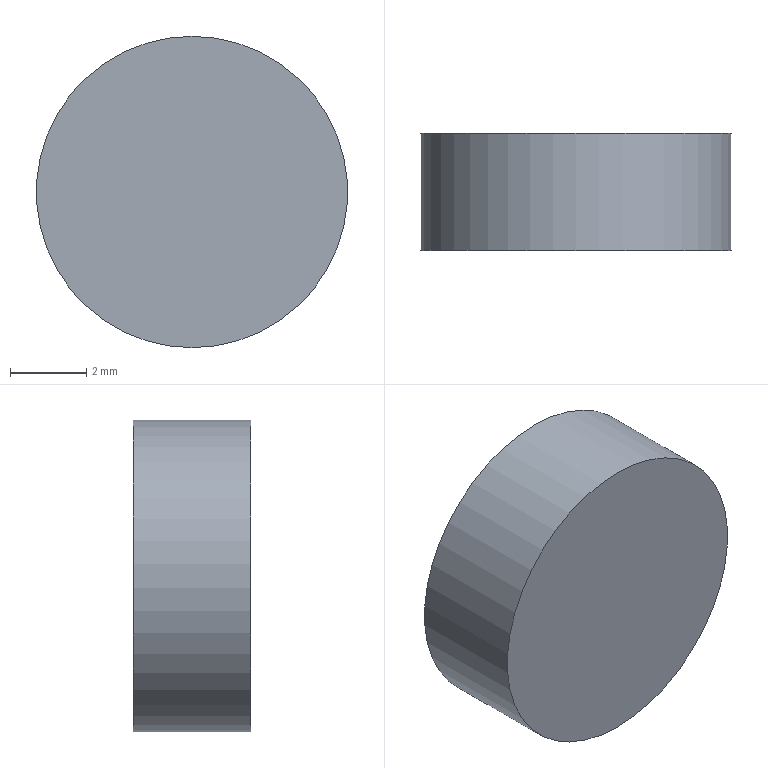Part | STEP file | 1_id362_x_t | 1 solid | 3 faces | box 8.17 x 3.075 x 8.17 mm | volume 161.205 mm3 | plane 2 | cylinder 1 | commonest cylinder face diameters 8.17 x1
STEP:
#1=CARTESIAN_POINT('',(0.,0.,0.));
#2=DIRECTION('',(0.,0.,1.));
#3=DIRECTION('',(1.,0.,0.));
#4=AXIS2_PLACEMENT_3D('',#1,#2,#3);
#5=CARTESIAN_POINT('',(734.725,165.025,-66.585));
#6=VERTEX_POINT('',#5);
#7=CARTESIAN_POINT('',(734.725,165.025,-70.67));
#8=DIRECTION('',(0.,-1.,0.));
#9=DIRECTION('',(0.,0.,1.));
#10=AXIS2_PLACEMENT_3D('',#7,#8,#9);
#11=CIRCLE('',#10,4.085);
#12=CARTESIAN_POINT('',(734.725,165.025,-70.67));
#13=DIRECTION('',(0.,1.,0.));
#14=DIRECTION('',(0.,0.,1.));
#15=AXIS2_PLACEMENT_3D('',#12,#13,#14);
#16=CYLINDRICAL_SURFACE('',#15,4.085);
#17=CARTESIAN_POINT('',(6.283,0.));
#18=DIRECTION('',(-1.,0.));
#19=VECTOR('',#18,1.);
#20=LINE('',#17,#19);
#21=(GEOMETRIC_REPRESENTATION_CONTEXT(2)PARAMETRIC_REPRESENTATION_CONTEXT()REPRESENTATION_CONTEXT('',''));
#22=DEFINITIONAL_REPRESENTATION('',(#20),#21);
#23=PCURVE('',#16,#22);
#24=CARTESIAN_POINT('',(734.725,165.025,-70.67));
#25=DIRECTION('',(0.,-1.,0.));
#26=DIRECTION('',(0.,0.,-1.));
#27=AXIS2_PLACEMENT_3D('',#24,#25,#26);
#28=PLANE('',#27);
#29=CARTESIAN_POINT('',(0.,0.));
#30=DIRECTION('',(-1.,0.));
#31=AXIS2_PLACEMENT_2D('',#29,#30);
#32=CIRCLE('',#31,4.085);
#33=(GEOMETRIC_REPRESENTATION_CONTEXT(2)PARAMETRIC_REPRESENTATION_CONTEXT()REPRESENTATION_CONTEXT('',''));
#34=DEFINITIONAL_REPRESENTATION('',(#32),#33);
#35=PCURVE('',#28,#34);
#36=SURFACE_CURVE('',#11,(#23,#35),.PCURVE_S1.);
#37=EDGE_CURVE('',#6,#6,#36,.T.);
#38=ORIENTED_EDGE('',*,*,#37,.F.);
#39=CARTESIAN_POINT('',(734.725,168.1,-66.585));
#40=VERTEX_POINT('',#39);
#41=CARTESIAN_POINT('',(734.725,165.025,-66.585));
#42=CARTESIAN_POINT('',(734.725,168.1,-66.585));
#43=B_SPLINE_CURVE_WITH_KNOTS('',1,(#41,#42),.UNSPECIFIED.,.F.,.F.,(2,2),(0.,3.075),.PIECEWISE_BEZIER_KNOTS.);
#44=CARTESIAN_POINT('',(6.283,0.));
#45=DIRECTION('',(0.,1.));
#46=VECTOR('',#45,1.);
#47=LINE('',#44,#46);
#48=(GEOMETRIC_REPRESENTATION_CONTEXT(2)PARAMETRIC_REPRESENTATION_CONTEXT()REPRESENTATION_CONTEXT('',''));
#49=DEFINITIONAL_REPRESENTATION('',(#47),#48);
#50=PCURVE('',#16,#49);
#51=CARTESIAN_POINT('',(0.,0.));
#52=DIRECTION('',(0.,1.));
#53=VECTOR('',#52,1.);
#54=LINE('',#51,#53);
#55=(GEOMETRIC_REPRESENTATION_CONTEXT(2)PARAMETRIC_REPRESENTATION_CONTEXT()REPRESENTATION_CONTEXT('',''));
#56=DEFINITIONAL_REPRESENTATION('',(#54),#55);
#57=PCURVE('',#16,#56);
#58=SEAM_CURVE('',#43,(#50,#57),.PCURVE_S1.);
#59=EDGE_CURVE('',#6,#40,#58,.T.);
#60=ORIENTED_EDGE('',*,*,#59,.T.);
#61=CARTESIAN_POINT('',(734.725,168.1,-70.67));
#62=DIRECTION('',(0.,-1.,0.));
#63=DIRECTION('',(0.,0.,1.));
#64=AXIS2_PLACEMENT_3D('',#61,#62,#63);
#65=CIRCLE('',#64,4.085);
#66=CARTESIAN_POINT('',(6.283,3.075));
#67=DIRECTION('',(-1.,0.));
#68=VECTOR('',#67,1.);
#69=LINE('',#66,#68);
#70=(GEOMETRIC_REPRESENTATION_CONTEXT(2)PARAMETRIC_REPRESENTATION_CONTEXT()REPRESENTATION_CONTEXT('',''));
#71=DEFINITIONAL_REPRESENTATION('',(#69),#70);
#72=PCURVE('',#16,#71);
#73=CARTESIAN_POINT('',(734.725,168.1,-70.67));
#74=DIRECTION('',(0.,-1.,0.));
#75=DIRECTION('',(0.,0.,-1.));
#76=AXIS2_PLACEMENT_3D('',#73,#74,#75);
#77=PLANE('',#76);
#78=CARTESIAN_POINT('',(0.,0.));
#79=DIRECTION('',(-1.,0.));
#80=AXIS2_PLACEMENT_2D('',#78,#79);
#81=CIRCLE('',#80,4.085);
#82=(GEOMETRIC_REPRESENTATION_CONTEXT(2)PARAMETRIC_REPRESENTATION_CONTEXT()REPRESENTATION_CONTEXT('',''));
#83=DEFINITIONAL_REPRESENTATION('',(#81),#82);
#84=PCURVE('',#77,#83);
#85=SURFACE_CURVE('',#65,(#72,#84),.PCURVE_S1.);
#86=EDGE_CURVE('',#40,#40,#85,.T.);
#87=ORIENTED_EDGE('',*,*,#86,.T.);
#88=ORIENTED_EDGE('',*,*,#59,.F.);
#89=EDGE_LOOP('',(#38,#60,#87,#88));
#90=FACE_BOUND('',#89,.T.);
#91=ADVANCED_FACE('',(#90),#16,.T.);
#92=ORIENTED_EDGE('',*,*,#37,.T.);
#93=EDGE_LOOP('',(#92));
#94=FACE_BOUND('',#93,.T.);
#95=ADVANCED_FACE('',(#94),#28,.T.);
#96=ORIENTED_EDGE('',*,*,#86,.F.);
#97=EDGE_LOOP('',(#96));
#98=FACE_BOUND('',#97,.T.);
#99=ADVANCED_FACE('',(#98),#77,.F.);
#100=CLOSED_SHELL('',(#91,#95,#99));
#101=MANIFOLD_SOLID_BREP('',#100);
#102=(LENGTH_UNIT()NAMED_UNIT(*)SI_UNIT(.MILLI.,.METRE.));
#103=UNCERTAINTY_MEASURE_WITH_UNIT(LENGTH_MEASURE(0.00001),#102,'','');
#104=(NAMED_UNIT(*)PLANE_ANGLE_UNIT()SI_UNIT($,.RADIAN.));
#105=(NAMED_UNIT(*)SI_UNIT($,.STERADIAN.)SOLID_ANGLE_UNIT());
#106=(GEOMETRIC_REPRESENTATION_CONTEXT(3)GLOBAL_UNCERTAINTY_ASSIGNED_CONTEXT((#103))GLOBAL_UNIT_ASSIGNED_CONTEXT((#102,#104,#105))REPRESENTATION_CONTEXT('',''));
#107=ADVANCED_BREP_SHAPE_REPRESENTATION('',(#4,#101),#106);